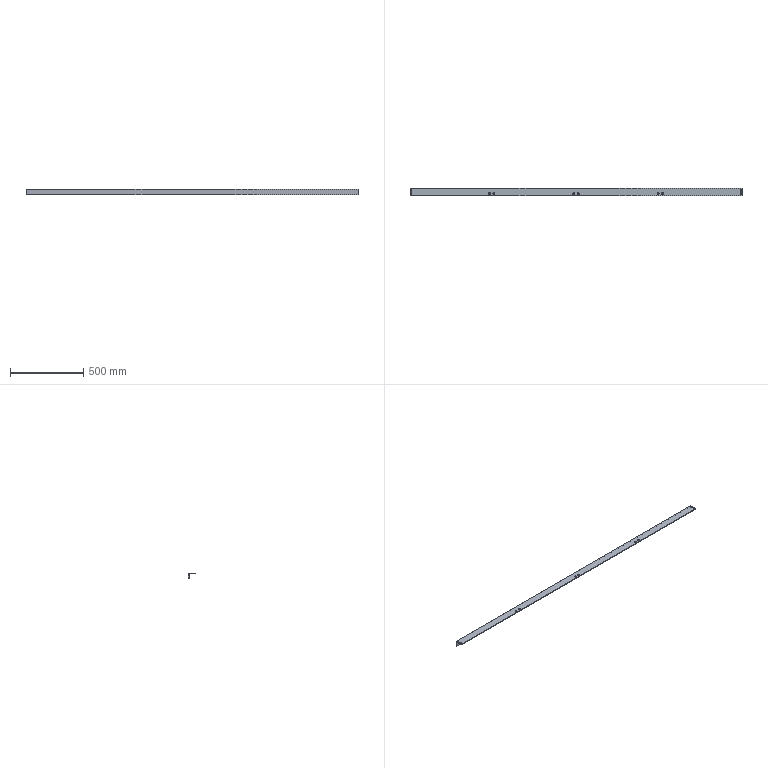Part | SolidWorks | features Extrusion 1, HoleWzd 1, ICE 1, WeldmentFeature 1 | 1 solid | 49 faces | box 2260 x 50 x 40 mm | volume 891378 mm3 | cone 20 | cylinder 20 | plane 9 | commonest cylinder face diameters 6.6 x20